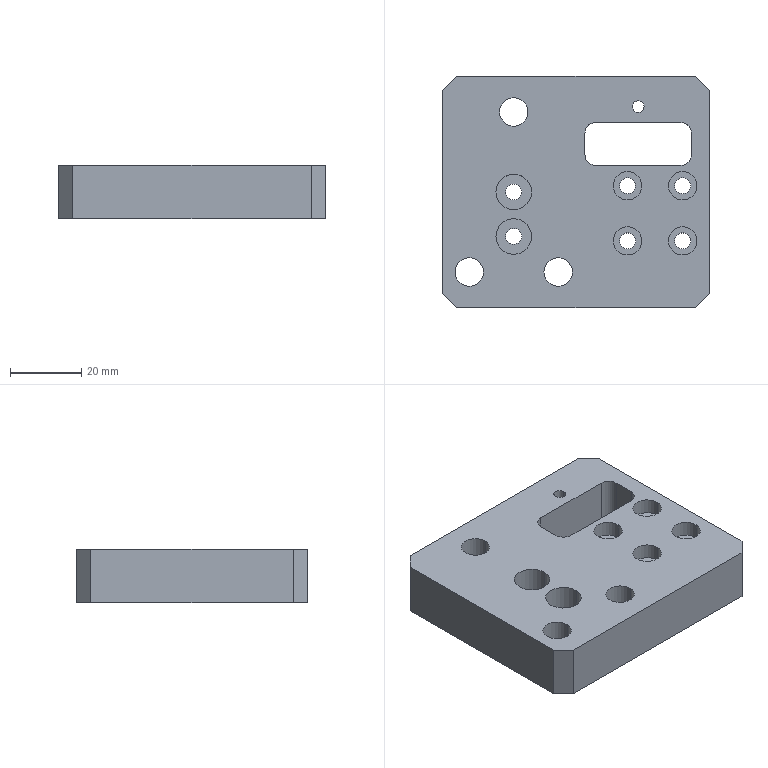Part | SolidWorks | features HoleWzd 4, Chamfer 1, Cut 1, Extrusion 1, Fillet 1, ICE 1 | 1 solid | 62 faces | box 75 x 65 x 15 mm | volume 61686 mm3 | cylinder 40 | plane 22 | commonest cylinder face diameters 8 x18 4.5 x12 6 x4 10 x4 3.3 x2